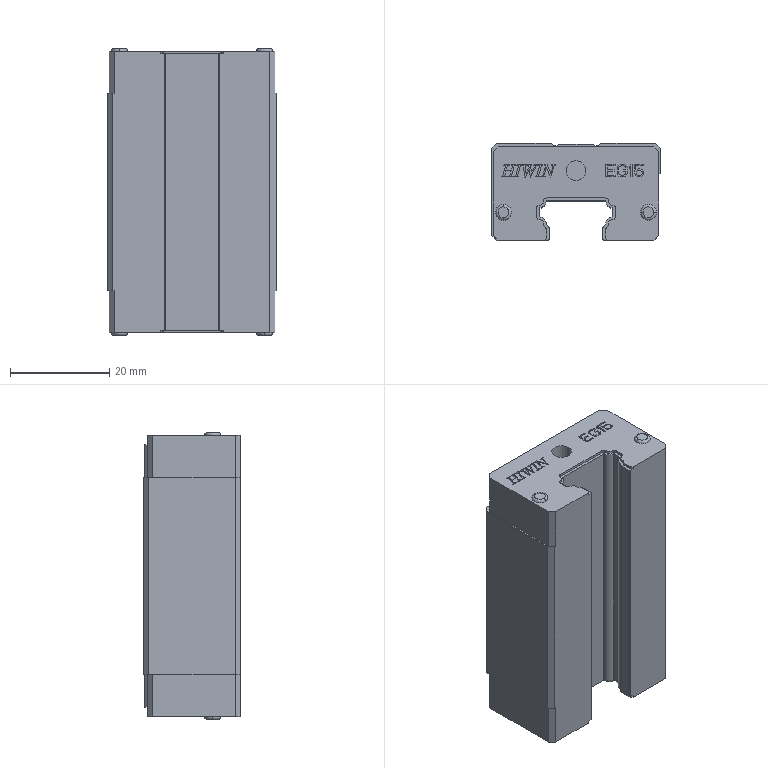Part | SolidWorks | features BaseBody 1 | 1 solid | 481 faces | box 34 x 19.5 x 57.8 mm | volume 30582 mm3 | plane 331 | spline 69 | cylinder 65 | torus 8 | cone 8 | commonest cylinder face diameters 1.6 x16 2.1 x12 0.46 x8 3.3 x8 3 x5 0.6 x4